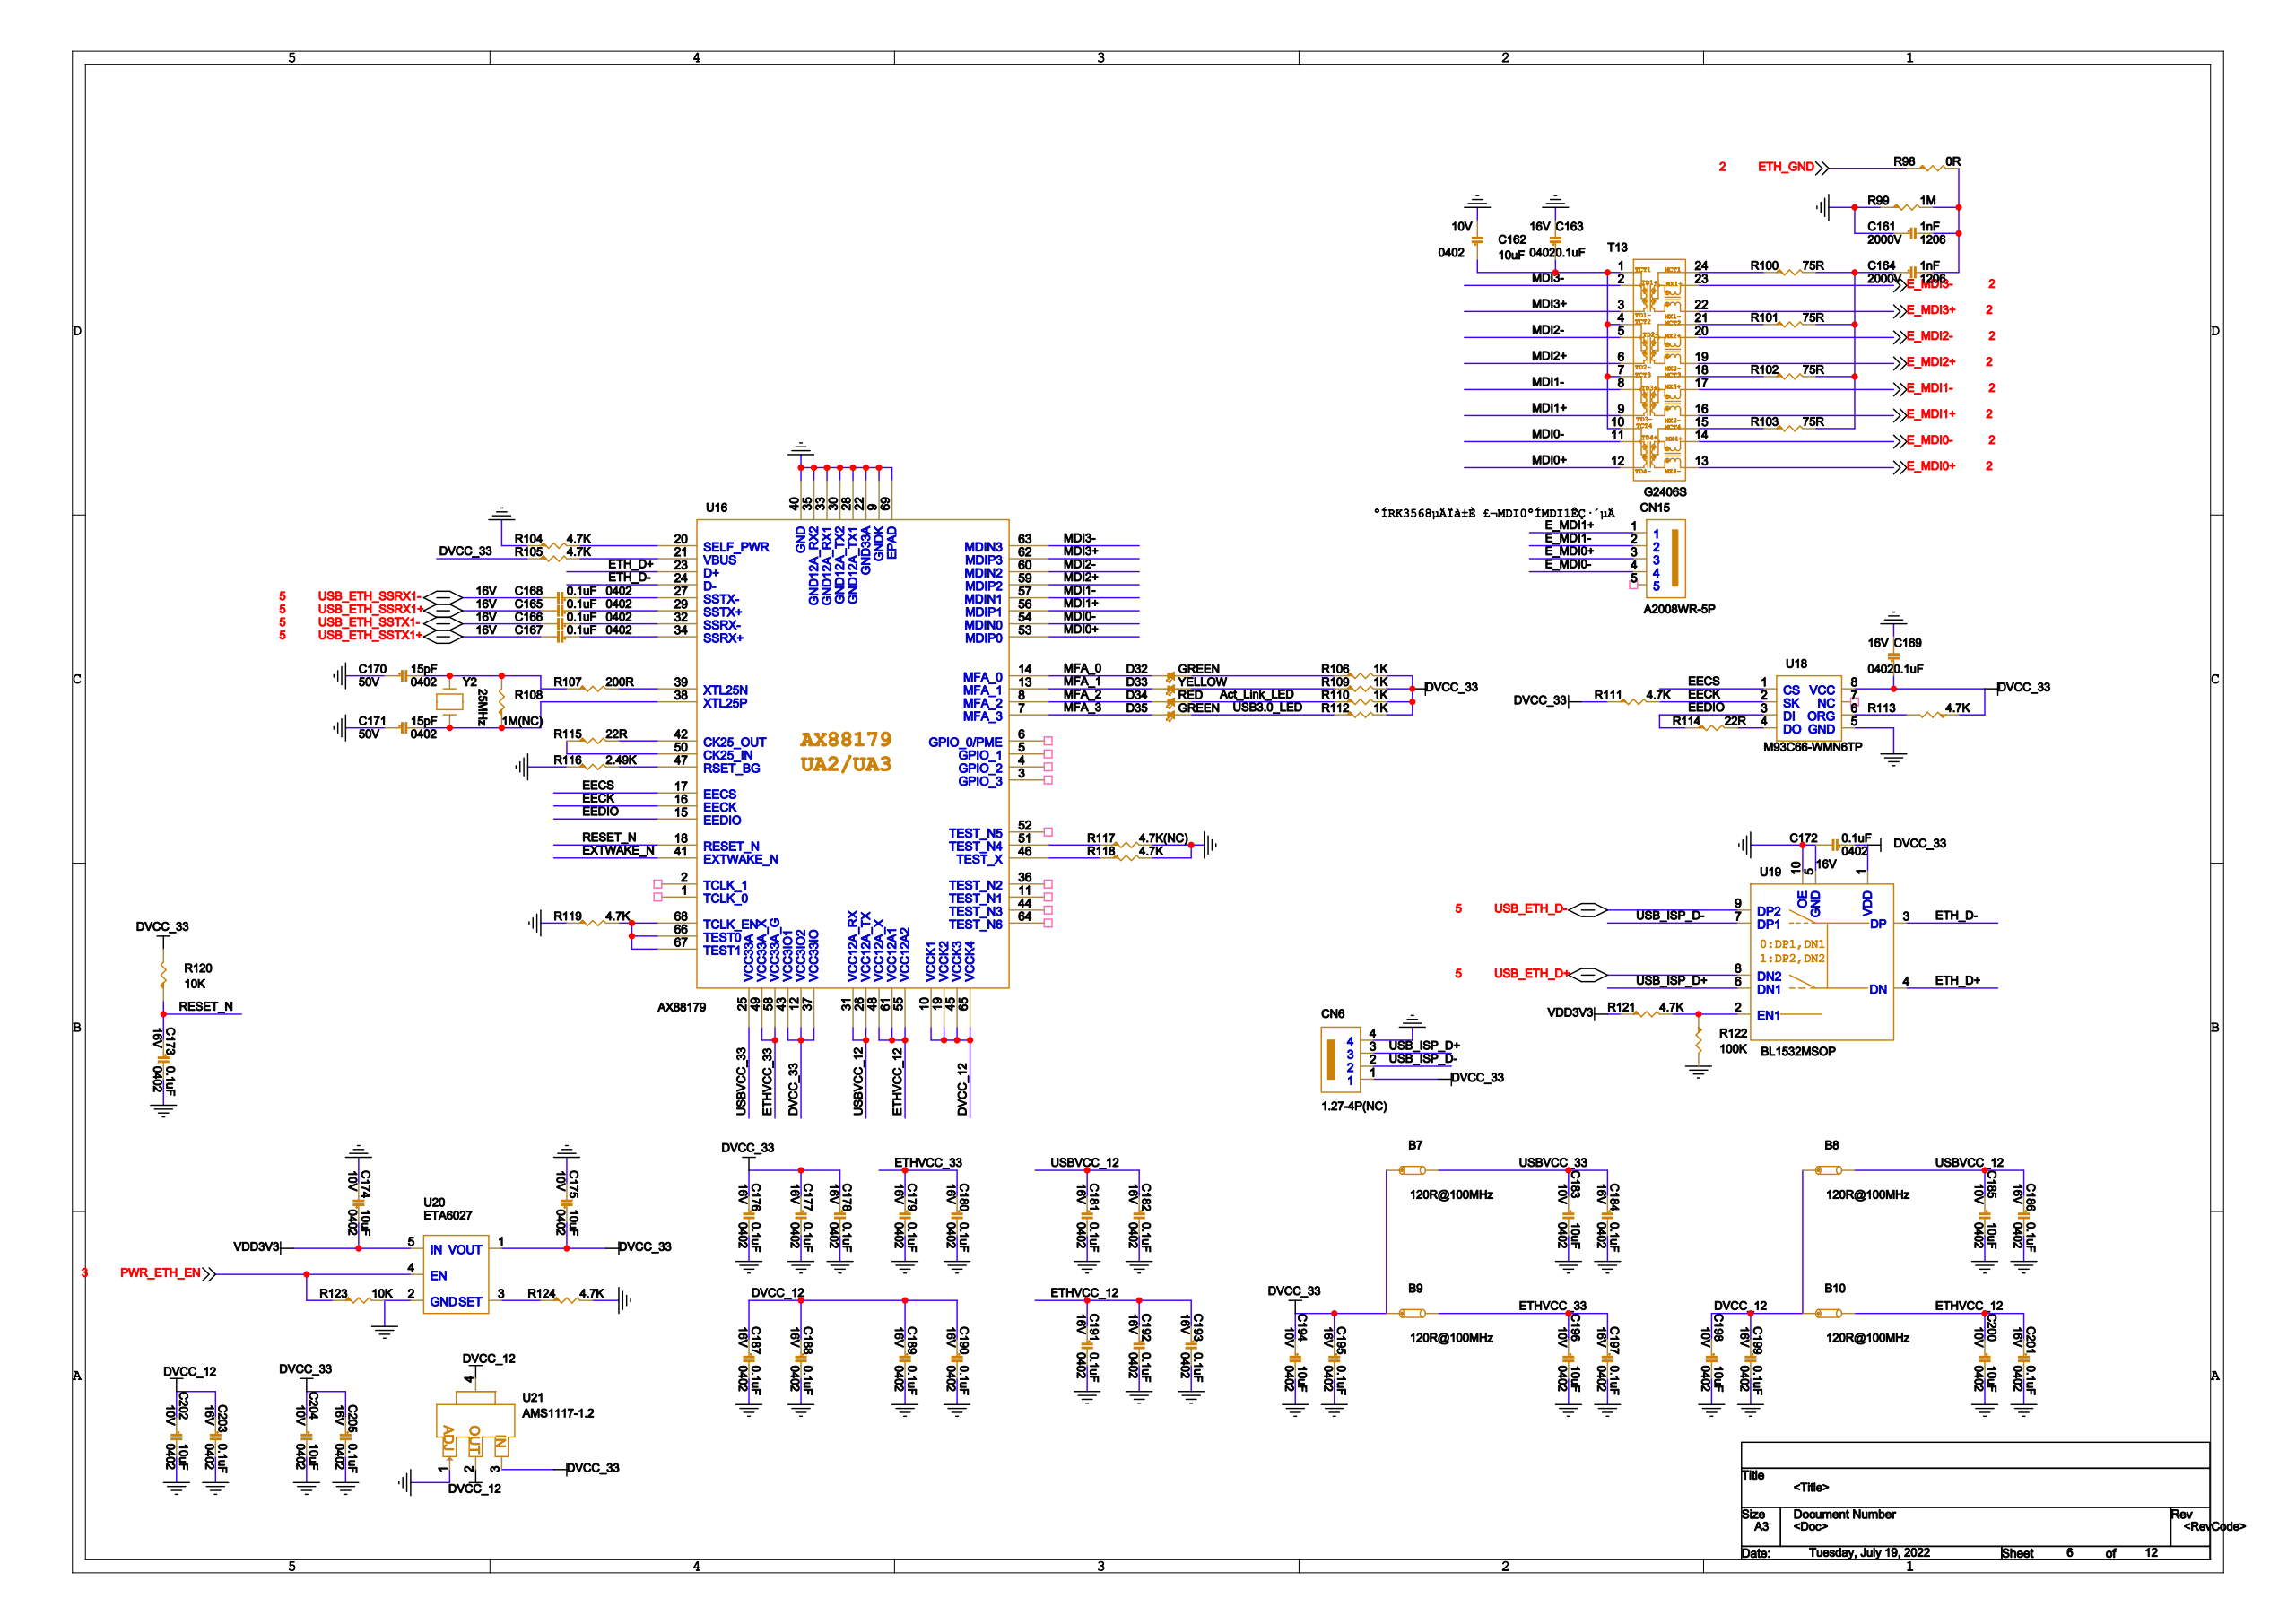Circuit board | Cadence Allegro | 970 parts | 627 nets | one sheet of the schematic
Parts on this sheet (reference | value | footprint):
B7 | 120R@100MHz | R0402
B8 | 120R@100MHz | R0402
B9 | 120R@100MHz | R0402
B10 | 120R@100MHz | R0402
C161 | 1nF | C1206
C162 | 10uF | C0402
C163 | 0.1uF | C0402
C164 | 1nF | C1206
C165 | 0.1uF | C0402
C166 | 0.1uF | C0402
C167 | 0.1uF | C0402
C168 | 0.1uF | C0402
C169 | 0.1uF | C0402
C170 | 15pF | C0402
C171 | 15pF | C0402
C172 | 0.1uF | C0402
C173 | 0.1uF | C0402
C174 | 10uF | C0402
C175 | 10uF | C0402
C176 | 0.1uF | C0402
C177 | 0.1uF | C0402
C178 | 0.1uF | C0402
C179 | 0.1uF | C0402
C180 | 0.1uF | C0402
C181 | 0.1uF | C0402
C182 | 0.1uF | C0402
C183 | 10uF | C0402
C184 | 0.1uF | C0402
C185 | 10uF | C0402
C186 | 0.1uF | C0402
C187 | 0.1uF | C0402
C188 | 0.1uF | C0402
C189 | 0.1uF | C0402
C190 | 0.1uF | C0402
C191 | 0.1uF | C0402
C192 | 0.1uF | C0402
C193 | 0.1uF | C0402
C194 | 10uF | C0402
C195 | 0.1uF | C0402
C196 | 10uF | C0402
C197 | 0.1uF | C0402
C198 | 10uF | C0402
C199 | 0.1uF | C0402
C200 | 10uF | C0402
C201 | 0.1uF | C0402
C202 | 10uF | C0402
C203 | 0.1uF | C0402
C204 | 10uF | C0402
C205 | 0.1uF | C0402
CN6 | 1.27-4P(NC) | SIP4_1P27
CN15 | A2008WR-5P | A2008WR_5P
D32 | GREEN | D0603
D33 | YELLOW | D0603
D34 | RED | D0603
D35 | GREEN | D0603
R98 | 0R | R0402
R99 | 1M | R1206
R100 | 75R | R0402
R101 | 75R | R0402
R102 | 75R | R0402
R103 | 75R | R0402
R104 | 4.7K | R0402
R105 | 4.7K | R0402
R106 | 1K | R0402
R107 | 200R | R0402
R108 | 1M(NC) | R0402
R109 | 1K | R0402
R110 | 1K | R0402
R111 | 4.7K | R0402
R112 | 1K | R0402
R113 | 4.7K | R0402
R114 | 22R | R0402
R115 | 22R | R0402
R116 | 2.49K | R0402
R117 | 4.7K(NC) | R0402
R118 | 4.7K | R0402
R119 | 4.7K | R0402
R120 | 10K | R0402
R121 | 4.7K | R0402
R122 | 100K | R0402
R123 | 10K | R0402
R124 | 4.7K | R0402
T13 | G2406S | G2406S
U16 | AX88179 | QFN68-0P4-A
U18 | M93C66-WMN6TP | SO8
U19 | BL1532MSOP | MSOP10
U20 | ETA6027 | SOT23-5
U21 | AMS1117-1.2 | SOT223
Y2 | 25MHz | X3225
Nets of these parts (net: part-pin ...):
VDD3V3: C174-1 R121-1 U20-5
GND: C161-1 C162-2 C163-2 C169-2 C170-1 C171-1 C172-2 C173-2 C174-2 C175-2 C176-2 C177-2 C178-2 C179-2 C180-2 C181-2 C182-2 C183-2 C184-2 C185-2 C186-2 C187-2 C188-2 C189-2 C190-2 C191-2 C192-2 C193-2 C194-2 C195-2 C196-2 C197-2 C198-2 C199-2 C200-2 C201-2 C202-2 C203-2 C204-2 C205-2 CN6-4 R99-1 R104-1 R116-1 R117-2 R118-2 R119-1 R122-2 R123-2 R124-2 U18-5 U19-5 U19-10 U20-2 U21-1 Y2-2 Y2-4 U16-9 U16-22 U16-28 U16-30 U16-33 U16-35 U16-40 U16-69
E_MDI1+: CN15-1 T13-16
E_MDI1-: CN15-2 T13-17
E_MDI0+: CN15-3 T13-13
E_MDI0-: CN15-4 T13-14
E_MDI3+: T13-22
E_MDI3-: T13-23
E_MDI2+: T13-19
E_MDI2-: T13-20
ETH_GND: R98-1
N19276442: C170-2 R107-1 R108-2 Y2-1
N19276451: C171-2 R108-1 Y2-3 U16-38
DVCC_12: B8-1 B10-1 C187-1 C188-1 C189-1 C190-1 C198-1 C199-1 C202-1 C203-1 U21-2 U21-4 U16-10 U16-19 U16-45 U16-65
ETHVCC_12: B10-2 C191-1 C192-1 C193-1 C200-1 C201-1 U16-48 U16-55 U16-61
DVCC_33: B7-1 B9-1 C169-1 C172-1 C175-1 C176-1 C177-1 C178-1 C194-1 C195-1 C204-1 C205-1 CN6-1 R105-1 R106-2 R109-2 R110-2 R111-1 R112-2 R113-1 R120-2 U18-8 U19-1 U20-1 U21-3 U16-12 U16-37 U16-43
USBVCC_33: B7-2 C183-1 C184-1 U16-25
USBVCC_12: B8-2 C181-1 C182-1 C185-1 C186-1 U16-26 U16-31
ETHVCC_33: B9-2 C179-1 C180-1 C196-1 C197-1 U16-49 U16-58
N19268831: C161-2 C164-2 R98-2 R99-2
N19268709: C164-1 R100-2 R101-2 R102-2 R103-2
USB_ISP_D-: CN6-2 U19-7
USB_ISP_D+: CN6-3 U19-6
N19284502: D32-1 R106-1
MFA_0: D32-2 U16-14
USB3.0_LED: D35-1 R112-1
MFA_3: D35-2 U16-7
N19284505: D33-1 R109-1
MFA_1: D33-2 U16-13
ACT_LINK_LED: D34-1 R110-1
MFA_2: D34-2 U16-8
N19274491: R121-2 R122-1 U19-2
N19268697: R103-1 T13-15
N19268706: R100-1 T13-24
N19268703: R101-1 T13-21
N19268700: R102-1 T13-18
N19269936: R104-2 U16-20
N19274186: R105-2 U16-21
EECK: R111-2 U18-2 U16-16
N19283441: R113-2 U18-6
N19284102: R118-1 U16-46
N19277254: R119-2 U16-66 U16-67 U16-68
N19270584: R124-1 U20-3
N19276042: R107-2 U16-39
EEDIO: R114-1 U18-3 U16-15
N19283407: R114-2 U18-4
N19277009: R115-1 U16-50
N19277014: R115-2 U16-42
N19277199: R116-2 U16-47
N19284099: R117-1 U16-51
RESET_N: C173-1 R120-1 U16-18
PWR_ETH_EN: R123-1 U20-4
N19268997: C162-1 C163-1 T13-1 T13-4 T13-7 T13-10
MDI3-: T13-2 U16-63
MDI3+: T13-3 U16-62
MDI2-: T13-5 U16-60
MDI2+: T13-6 U16-59
MDI1-: T13-8 U16-57
MDI1+: T13-9 U16-56
MDI0-: T13-11 U16-54
MDI0+: T13-12 U16-53
ETH_D+: U19-4 U16-23
USB_ETH_D+: U19-8
ETH_D-: U19-3 U16-24
USB_ETH_D-: U19-9
USB_ETH_SSRX1+: C165-2
USB_ETH_SSRX1-: C168-2
USB_ETH_SSTX1+: C167-2
USB_ETH_SSTX1-: C166-2
EECS: U18-1 U16-17
EXTWAKE_N: U16-41
N19275233: C167-1 U16-34
N19275230: C166-1 U16-32
N19275227: C165-1
N19275164: C168-1 U16-27